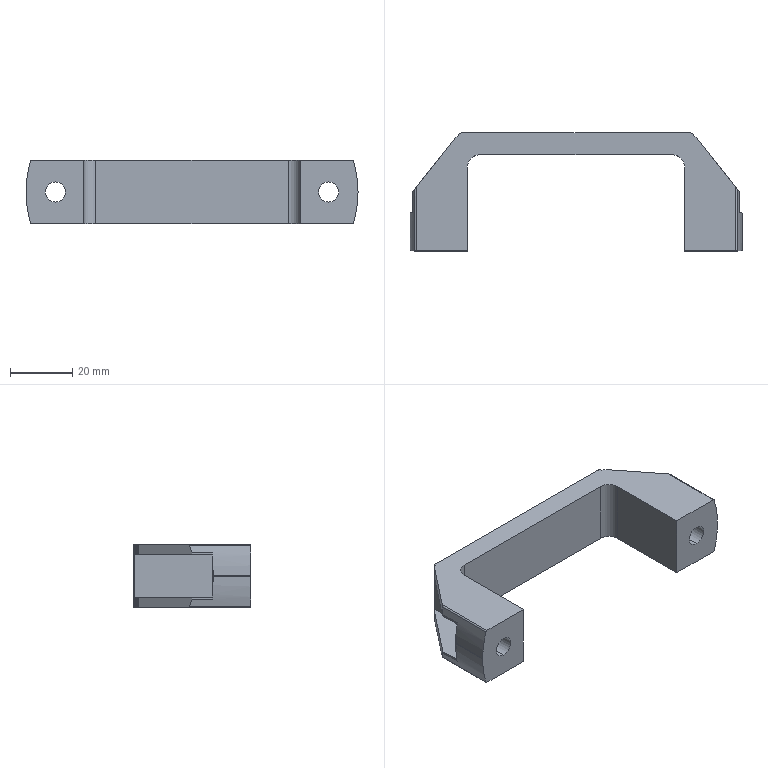Part | SolidWorks | features BaseBody 1 | 1 solid | 65 faces | box 107 x 38 x 20.5 mm | volume 23344 mm3 | plane 40 | cylinder 25 | commonest cylinder face diameters 1 x9 6.5 x4 12.5 x4 68.166 x4 4 x2 8 x2